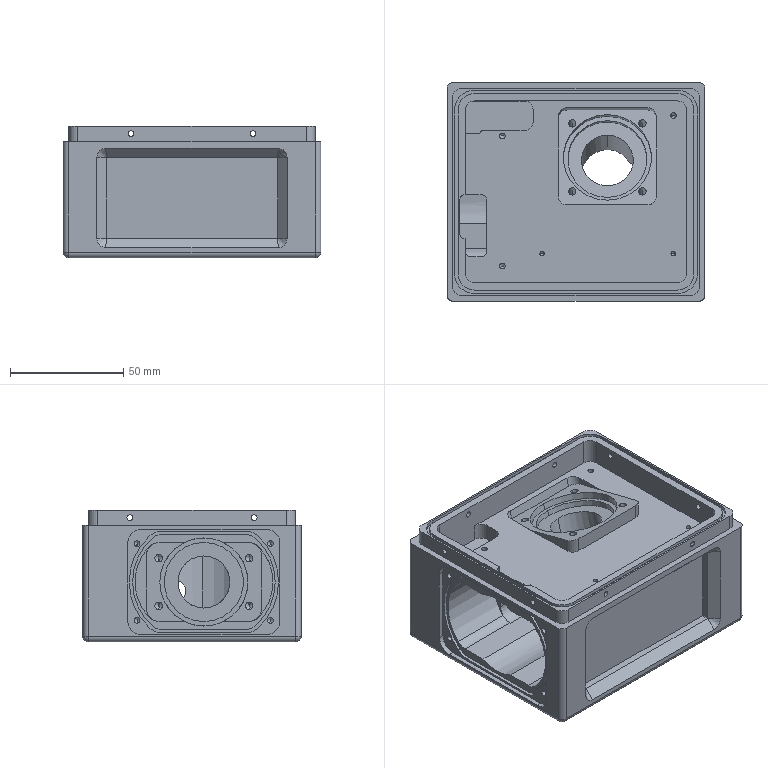Part | SolidWorks | features 3DProfileFeature 13, HoleWzd 13, Cut 10, Fillet 10, LPattern 9, SketchHole 7, Chamfer 3, MirrorPattern 3, Boss 2, VarFillet 2, Extrusion 1, RefAxis 1, RevCut 1 | 1 solid | 313 faces | box 114 x 96.5 x 58.3 mm | volume 315384 mm3 | cylinder 161 | plane 93 | cone 46 | spline 9 | sphere 4 | commonest cylinder face diameters 2.5 x30 3.3 x16 12 x16 8 x14 5 x13 0.4 x8